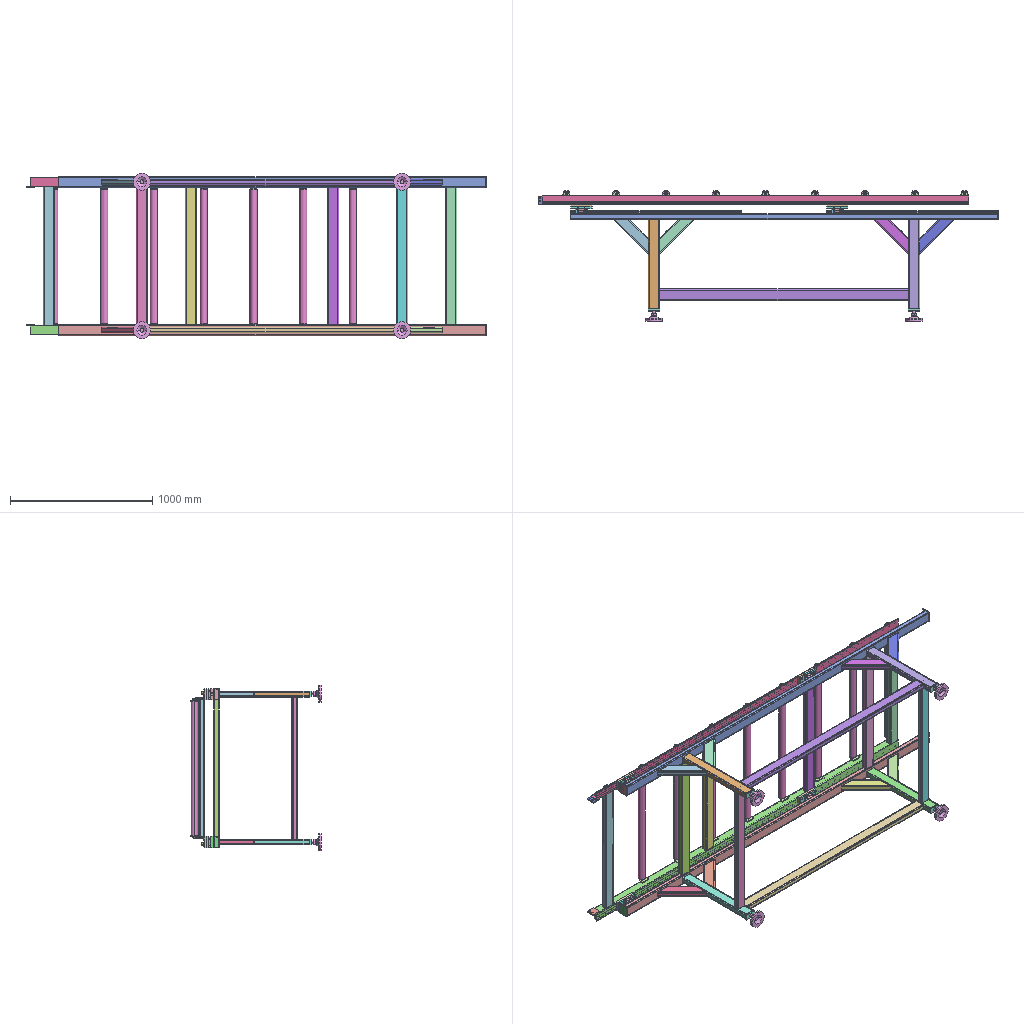Assembly | SolidWorks | 15 different items | 57 placed | box 3235 x 919 x 1161 mm
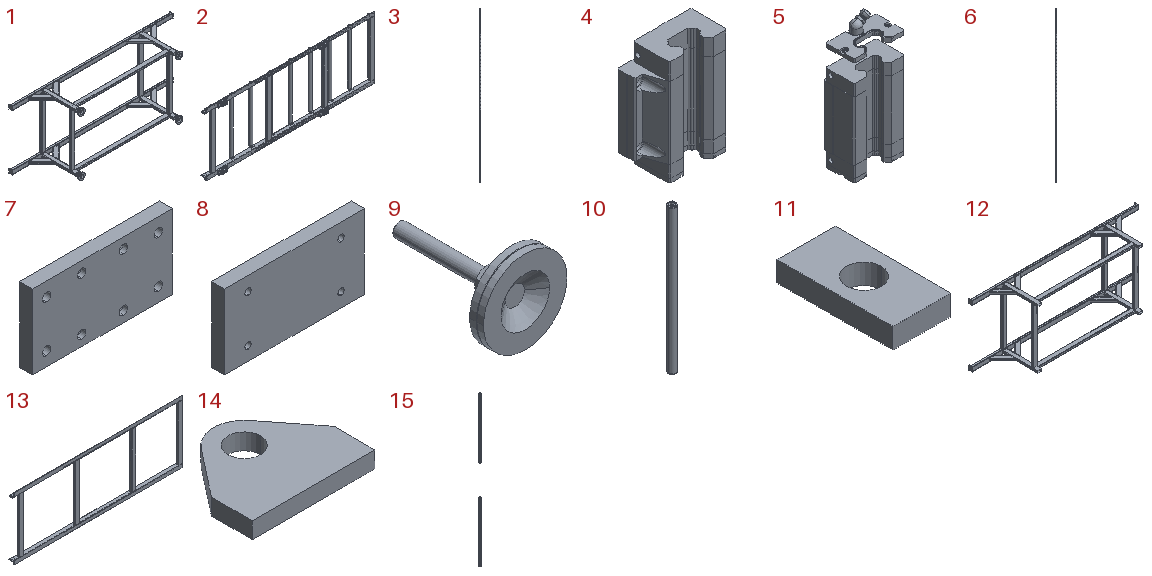Parts list (item | name | quantity | parent item | size | volume | features):
1 | (subassembly) | x1 | - | 3010 x 778.6 x 1163 mm | 17961198 mm3 | features ReferencePattern 6, LocalLPattern 2
2 | (subassembly) | x1 | - | - | 28545845 mm3 | features ReferencePattern 33, LocalLPattern 3
3 | (subassembly) | x2 | in 2 | 20 x 17.5 x 3000 mm | 901599 mm3 | features LocalLPattern 1, ReferencePattern 1
4 | - | x4 | in 2 | 70 x 30.5 x 84.75 mm | 108873 mm3 | features ICE 25, Extrusion 5, MirrorPattern 5, Fillet 4, MirrorSolid 4, Chamfer 3, RevCut 3, Dome 2, LPattern 2, Revolution 2, DeleteBody 1, LibraryFeature 1
5 | - | x1 | in 3 | 44 x 25.71 x 103.7 mm | 65250 mm3 | features ICE 23, Extrusion 5, MirrorPattern 5, Fillet 4, MirrorSolid 4, Chamfer 3, Dome 2, Revolution 2, LibraryFeature 1, RevCut 1
6 | - | x2 | in 3 | 20 x 17.5 x 3000 mm | 901599 mm3 | features ICE 15, Chamfer 3, Extrusion 3, Fillet 3, MirrorPattern 3, MirrorSolid 3, RevCut 3, LPattern 2, DeleteBody 1, Dome 1
7 | - | x4 | in 2 | 150 x 14 x 80 mm | 156803 mm3 | features HoleWzd 2, Extrusion 1
8 | - | x4 | in 2 | 150 x 14 x 80 mm | 165966 mm3 | features Extrusion 1, HoleWzd 1
9 | - | x4 | in 1 | 120 x 181 x 120 mm | 289918 mm3 | features ICE 2, RevCut 2, Chamfer 1, Revolution 1
10 | - | x9 | in 2 | 50 x 50 x 985 mm | 1880684 mm3 | features Chamfer 2, ICE 2, Revolution 1
11 | - | x4 | in 1 | 40 x 80 x 14 mm | 38467 mm3 | features Extrusion 1
12 | - | x1 | in 1 | 3010 x 690 x 1120 mm | 15558930 mm3 | features ICE 2, WeldCornerFeat 2, 3DProfileFeature 1, WeldMemberFeat 1, WeldmentFeature 1
13 | - | x1 | in 2 | 3030 x 63 x 1106 mm | 7792453 mm3 | features ICE 4, WeldMemberFeat 3, 3DProfileFeature 1, HoleWzd 1, LPattern 1, WeldmentFeature 1
14 | - | x18 | in 2 | 60 x 49 x 8 mm | 16525 mm3 | features Extrusion 1
15 | - | x1 | in 1 | 23.859 x 22 x 3000 mm | 1088729 mm3 | features Chamfer 1, Extrusion 1, HoleWzd 1, ICE 1, LPattern 1
Mates (type | each side: item.copy, entity, surface, feature):
In the top assembly
Concentric | assembly face | assembly face | 4 times
LimitDistanceDim | 12.1 face plane Rectangular tube 80 X 40 X 4.0(1) | assembly face
DistanceDim | 7.1 face plane Boss-Extrude1 | 12.1 face plane Rectangular tube 80 X 40 X 4.0(1)
Width | 4.1 face plane Cut-Extrude11 | 4.1 face plane Cut-Extrude11 | 15.1 face plane Boss-Extrude1 | 15.1 face plane Boss-Extrude1
DistanceDim | assembly face | 13.1 face plane Equal angle 6.3X6(1)
Width | assembly face | assembly face | 6.1 face plane Boss-Extrude8 | 6.1 face plane Boss-Extrude8
In subassembly 1
Coincident | 12.2 face plane Rectangular tube 80 X 40 X 4.0(1) | 1.1 face | 2 times
Width | 1.1 face | 1.1 face | 12.2 face plane Rectangular tube 80 X 40 X 4.0(1) | 12.2 face plane Rectangular tube 80 X 40 X 4.0(1)
DistanceDim | 9.1 face plane Boss-Extrude2 | 11.1 face plane Boss-Extrude1
Concentric | 9.1 face cylinder Revolve1 | 11.1 face cylinder Boss-Extrude1
Coincident | 12.2 face plane Rectangular tube 80 X 40 X 4.0(1) | 11.1 face plane Boss-Extrude1 | 3 times
Coincident | 12.2 face plane Rectangular tube 80 X 40 X 4.0(1) | 15.2 face plane Boss-Extrude1 | 2 times
Width | 15.2 face plane Boss-Extrude1 | 15.2 face plane Boss-Extrude1 | 12.2 face plane Rectangular tube 80 X 40 X 4.0(1) | 12.2 face plane Rectangular tube 80 X 40 X 4.0(1)
In subassembly 2
Coincident | 13.2 face plane Equal angle 6.3X6(1) | 14.1 face plane Boss-Extrude1
DistanceDim | 13.2 face plane Equal angle 6.3X6(1) | 14.1 face plane Boss-Extrude1
DistanceDim | 14.1 face plane Boss-Extrude1 | 13.2 face plane Equal angle 6.3X6(1)
Coincident | 13.2 face plane Equal angle 6.3X6(1) | 14.2 face plane Boss-Extrude1
Coincident | 14.1 face plane Boss-Extrude1 | 14.2 face plane Boss-Extrude1
Concentric | 14.1 face cylinder Boss-Extrude1 | 14.2 face cylinder Boss-Extrude1
Concentric | 14.1 face cylinder Boss-Extrude1 | 10.1 face cylinder Revolve1
Coincident | 14.1 face plane Boss-Extrude1 | 10.1 face plane Revolve1
Coincident | 7.2 face plane Boss-Extrude1 | 8.1 face plane Boss-Extrude1 | 3 times
Coincident | 7.2 face plane Boss-Extrude1 | 2.1 face
Concentric | 7.2 face cylinder Hole size (% by) socket head cap screw type1 | 2.1 face
Coincident | 13.2 face plane Equal angle 6.3X6(1) | 8.1 face plane Boss-Extrude1
DistanceDim | 7.2 face plane Boss-Extrude1 | 13.2 face plane Equal angle 6.3X6(1)
Coincident | 13.2 face plane Equal angle 6.3X6(1) | 2.1 face | 16 times
DistanceDim | 2.1 face | 2.1 face
Coincident | 2.1 face | 2.1 face | 5 times
DistanceDim | 2.1 face | 13.2 face plane Equal angle 6.3X6(1)
Coincident | 7.2 face plane Boss-Extrude1 | 4.2 face plane Boss-Extrude1
Concentric | 7.2 face cylinder Hole size (% by) socket head cap screw type1 | 4.2 face cylinder Mirror1
Concentric | 7.2 face cylinder Hole size (% by) socket head cap screw type1 | 4.2 face cylinder Mirror2
Coincident | 13.2 face plane Equal angle 6.3X6(1) | 6.2 face plane Boss-Extrude8
Coincident | 2.1 face | 6.2 face plane Boss-Extrude8
DistanceDim | 13.2 face plane Equal angle 6.3X6(1) | 6.2 face plane Boss-Extrude8
Coincident | 13.2 face plane Equal angle 6.3X6(1) | 6.3 face plane Boss-Extrude8
DistanceDim | 13.2 face plane Equal angle 6.3X6(1) | 6.3 face plane Boss-Extrude8
Coincident | 2.1 face | 6.3 face plane Boss-Extrude8
DistanceDim | 8.1 face plane Boss-Extrude1 | 13.2 face plane Equal angle 6.3X6(1)
In subassembly 3
Coincident | 5.1 face | 6.4 face plane Boss-Extrude8 | 2 times
Path | 5.1 select_type:0 | 6.4 select_type:0